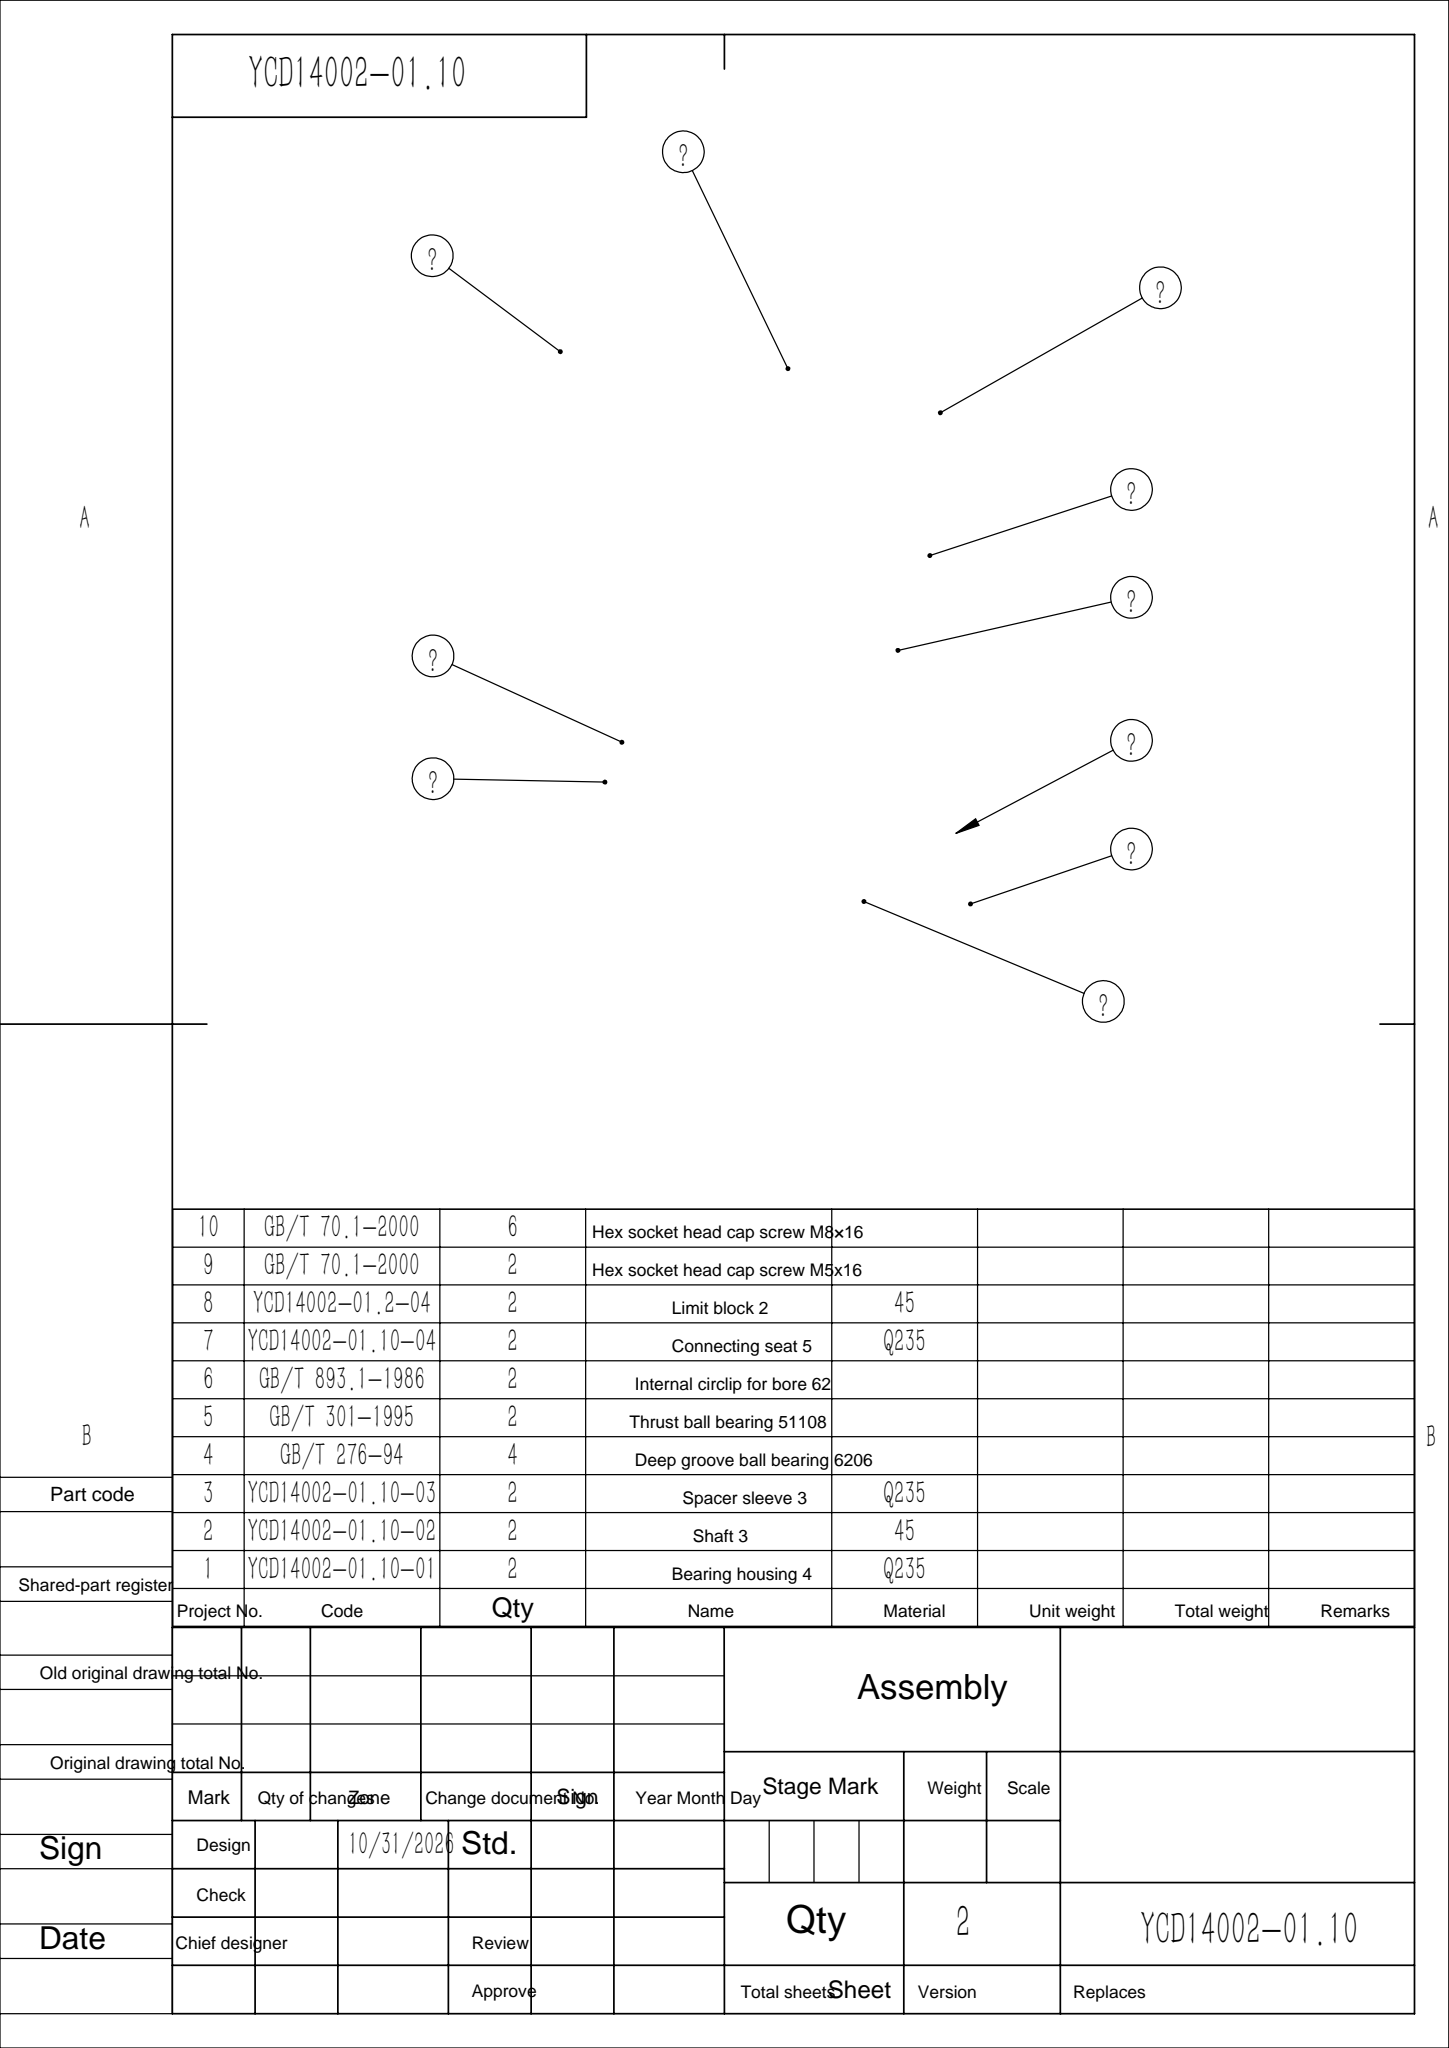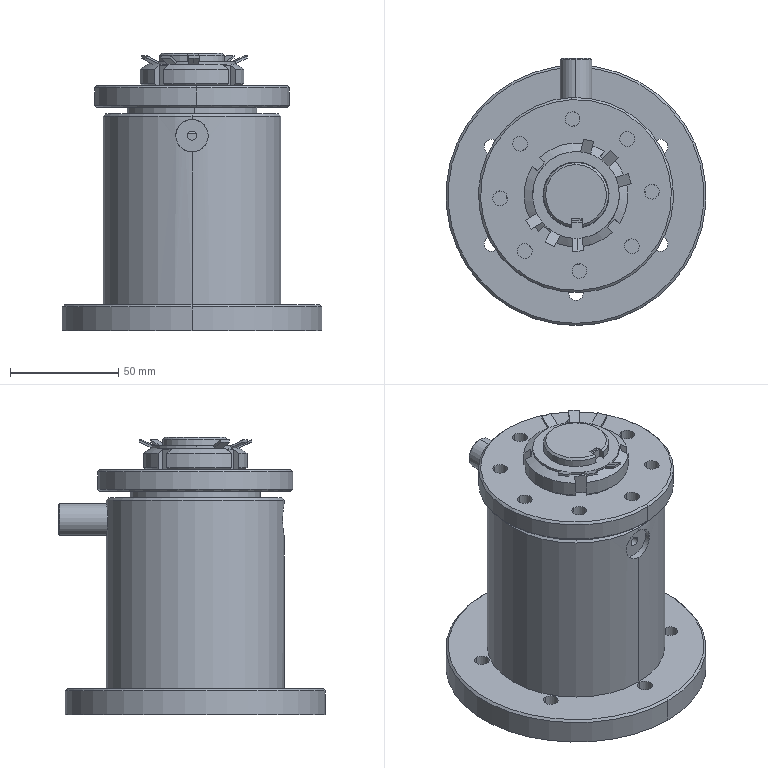Part | SolidWorks | 12 solids | 662 faces | box 120 x 123 x 128 mm | volume 584143 mm3 | sphere 186 | cylinder 151 | plane 133 | torus 132 | cone 60 | commonest cylinder face diameters 6.8 x28 40 x13 30 x12 62 x10 40.8 x8 52.2 x8